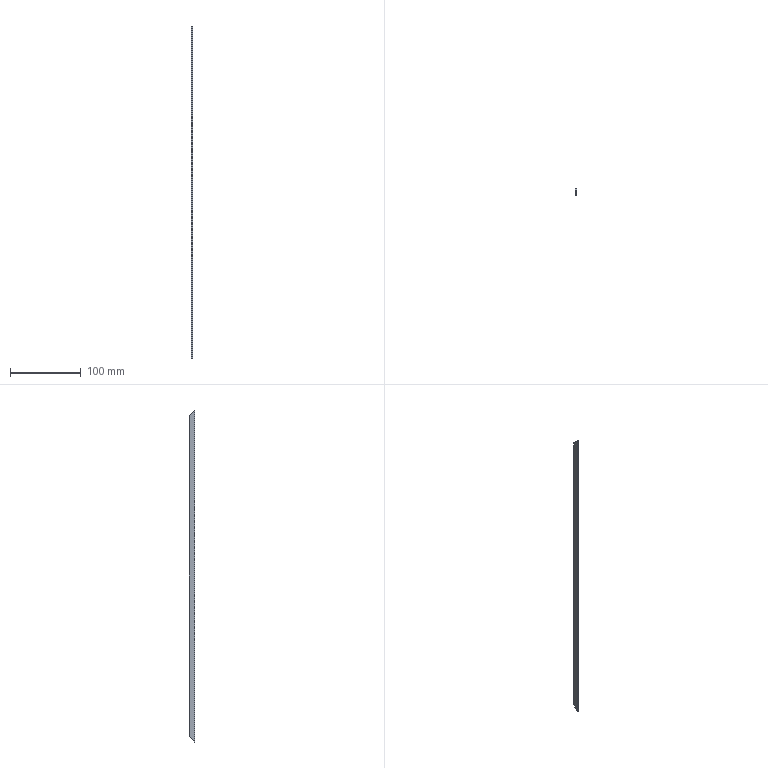Part | NX | features BREP 1 | 1 solid | 6 faces | box 1.5 x 8 x 468.1 mm | volume 5521 mm3 | plane 6
STEP:
#1=CARTESIAN_POINT('',(0.,8.,226.05));
#2=VERTEX_POINT('',#1);
#3=CARTESIAN_POINT('',(0.,8.,-226.05));
#4=VERTEX_POINT('',#3);
#5=CARTESIAN_POINT('',(0.,8.,234.05));
#6=DIRECTION('',(0.,0.,-1.));
#7=VECTOR('',#6,1000.);
#8=LINE('',#5,#7);
#9=EDGE_CURVE('',#2,#4,#8,.T.);
#10=ORIENTED_EDGE('',*,*,#9,.T.);
#11=CARTESIAN_POINT('',(0.,0.,-234.05));
#12=VERTEX_POINT('',#11);
#13=CARTESIAN_POINT('',(0.,8.,-226.05));
#14=DIRECTION('',(0.,-0.7071,-0.7071));
#15=VECTOR('',#14,1000.);
#16=LINE('',#13,#15);
#17=EDGE_CURVE('',#4,#12,#16,.T.);
#18=ORIENTED_EDGE('',*,*,#17,.T.);
#19=CARTESIAN_POINT('',(0.,0.,234.05));
#20=VERTEX_POINT('',#19);
#21=CARTESIAN_POINT('',(0.,0.,234.05));
#22=DIRECTION('',(0.,0.,-1.));
#23=VECTOR('',#22,1000.);
#24=LINE('',#21,#23);
#25=EDGE_CURVE('',#20,#12,#24,.T.);
#26=ORIENTED_EDGE('',*,*,#25,.F.);
#27=CARTESIAN_POINT('',(0.,0.,234.05));
#28=DIRECTION('',(0.,0.7071,-0.7071));
#29=VECTOR('',#28,1000.);
#30=LINE('',#27,#29);
#31=EDGE_CURVE('',#20,#2,#30,.T.);
#32=ORIENTED_EDGE('',*,*,#31,.T.);
#33=EDGE_LOOP('',(#10,#18,#26,#32));
#34=FACE_BOUND('',#33,.T.);
#35=CARTESIAN_POINT('',(0.,0.,234.05));
#36=DIRECTION('',(1.,0.,0.));
#37=DIRECTION('',(0.,1.,0.));
#38=AXIS2_PLACEMENT_3D('',#35,#36,#37);
#39=PLANE('',#38);
#40=ADVANCED_FACE('',(#34),#39,.F.);
#41=CARTESIAN_POINT('',(1.5,0.,-234.05));
#42=VERTEX_POINT('',#41);
#43=CARTESIAN_POINT('',(0.,0.,-234.05));
#44=DIRECTION('',(1.,0.,0.));
#45=VECTOR('',#44,1000.);
#46=LINE('',#43,#45);
#47=EDGE_CURVE('',#12,#42,#46,.T.);
#48=ORIENTED_EDGE('',*,*,#47,.T.);
#49=CARTESIAN_POINT('',(1.5,0.,234.05));
#50=VERTEX_POINT('',#49);
#51=CARTESIAN_POINT('',(1.5,0.,234.05));
#52=DIRECTION('',(0.,0.,-1.));
#53=VECTOR('',#52,1000.);
#54=LINE('',#51,#53);
#55=EDGE_CURVE('',#50,#42,#54,.T.);
#56=ORIENTED_EDGE('',*,*,#55,.F.);
#57=CARTESIAN_POINT('',(0.,0.,234.05));
#58=DIRECTION('',(1.,0.,0.));
#59=VECTOR('',#58,1000.);
#60=LINE('',#57,#59);
#61=EDGE_CURVE('',#20,#50,#60,.T.);
#62=ORIENTED_EDGE('',*,*,#61,.F.);
#63=ORIENTED_EDGE('',*,*,#25,.T.);
#64=EDGE_LOOP('',(#48,#56,#62,#63));
#65=FACE_BOUND('',#64,.T.);
#66=CARTESIAN_POINT('',(0.,0.,234.05));
#67=DIRECTION('',(0.,1.,0.));
#68=DIRECTION('',(1.,0.,0.));
#69=AXIS2_PLACEMENT_3D('',#66,#67,#68);
#70=PLANE('',#69);
#71=ADVANCED_FACE('',(#65),#70,.F.);
#72=ORIENTED_EDGE('',*,*,#55,.T.);
#73=CARTESIAN_POINT('',(1.5,8.,-226.05));
#74=VERTEX_POINT('',#73);
#75=CARTESIAN_POINT('',(1.5,8.,-226.05));
#76=DIRECTION('',(0.,0.7071,0.7071));
#77=VECTOR('',#76,1000.);
#78=LINE('',#75,#77);
#79=EDGE_CURVE('',#42,#74,#78,.T.);
#80=ORIENTED_EDGE('',*,*,#79,.T.);
#81=CARTESIAN_POINT('',(1.5,8.,226.05));
#82=VERTEX_POINT('',#81);
#83=CARTESIAN_POINT('',(1.5,8.,234.05));
#84=DIRECTION('',(0.,0.,-1.));
#85=VECTOR('',#84,1000.);
#86=LINE('',#83,#85);
#87=EDGE_CURVE('',#82,#74,#86,.T.);
#88=ORIENTED_EDGE('',*,*,#87,.F.);
#89=CARTESIAN_POINT('',(1.5,0.,234.05));
#90=DIRECTION('',(0.,-0.7071,0.7071));
#91=VECTOR('',#90,1000.);
#92=LINE('',#89,#91);
#93=EDGE_CURVE('',#82,#50,#92,.T.);
#94=ORIENTED_EDGE('',*,*,#93,.T.);
#95=EDGE_LOOP('',(#72,#80,#88,#94));
#96=FACE_BOUND('',#95,.T.);
#97=CARTESIAN_POINT('',(1.5,0.,234.05));
#98=DIRECTION('',(-1.,0.,0.));
#99=DIRECTION('',(0.,0.,1.));
#100=AXIS2_PLACEMENT_3D('',#97,#98,#99);
#101=PLANE('',#100);
#102=ADVANCED_FACE('',(#96),#101,.F.);
#103=ORIENTED_EDGE('',*,*,#87,.T.);
#104=CARTESIAN_POINT('',(0.,8.,-226.05));
#105=DIRECTION('',(-1.,0.,0.));
#106=VECTOR('',#105,1000.);
#107=LINE('',#104,#106);
#108=EDGE_CURVE('',#74,#4,#107,.T.);
#109=ORIENTED_EDGE('',*,*,#108,.T.);
#110=ORIENTED_EDGE('',*,*,#9,.F.);
#111=CARTESIAN_POINT('',(0.,8.,226.05));
#112=DIRECTION('',(1.,0.,0.));
#113=VECTOR('',#112,1000.);
#114=LINE('',#111,#113);
#115=EDGE_CURVE('',#2,#82,#114,.T.);
#116=ORIENTED_EDGE('',*,*,#115,.T.);
#117=EDGE_LOOP('',(#103,#109,#110,#116));
#118=FACE_BOUND('',#117,.T.);
#119=CARTESIAN_POINT('',(0.,8.,234.05));
#120=DIRECTION('',(0.,-1.,0.));
#121=DIRECTION('',(0.,0.,-1.));
#122=AXIS2_PLACEMENT_3D('',#119,#120,#121);
#123=PLANE('',#122);
#124=ADVANCED_FACE('',(#118),#123,.F.);
#125=ORIENTED_EDGE('',*,*,#79,.F.);
#126=ORIENTED_EDGE('',*,*,#47,.F.);
#127=ORIENTED_EDGE('',*,*,#17,.F.);
#128=ORIENTED_EDGE('',*,*,#108,.F.);
#129=EDGE_LOOP('',(#125,#126,#127,#128));
#130=FACE_BOUND('',#129,.T.);
#131=CARTESIAN_POINT('',(0.,8.,-226.05));
#132=DIRECTION('',(0.,0.7071,-0.7071));
#133=DIRECTION('',(-1.,0.,0.));
#134=AXIS2_PLACEMENT_3D('',#131,#132,#133);
#135=PLANE('',#134);
#136=ADVANCED_FACE('',(#130),#135,.T.);
#137=ORIENTED_EDGE('',*,*,#93,.F.);
#138=ORIENTED_EDGE('',*,*,#115,.F.);
#139=ORIENTED_EDGE('',*,*,#31,.F.);
#140=ORIENTED_EDGE('',*,*,#61,.T.);
#141=EDGE_LOOP('',(#137,#138,#139,#140));
#142=FACE_BOUND('',#141,.T.);
#143=CARTESIAN_POINT('',(0.,0.,234.05));
#144=DIRECTION('',(0.,-0.7071,-0.7071));
#145=DIRECTION('',(0.,0.7071,-0.7071));
#146=AXIS2_PLACEMENT_3D('',#143,#144,#145);
#147=PLANE('',#146);
#148=ADVANCED_FACE('',(#142),#147,.F.);
#149=CLOSED_SHELL('',(#40,#71,#102,#124,#136,#148));
#150=MANIFOLD_SOLID_BREP('',#149);
#151=(LENGTH_UNIT()NAMED_UNIT(*)SI_UNIT(.MILLI.,.METRE.));
#152=UNCERTAINTY_MEASURE_WITH_UNIT(LENGTH_MEASURE(0.00001),#151,'','');
#153=(NAMED_UNIT(*)PLANE_ANGLE_UNIT()SI_UNIT($,.RADIAN.));
#154=(NAMED_UNIT(*)SI_UNIT($,.STERADIAN.)SOLID_ANGLE_UNIT());
#155=(GEOMETRIC_REPRESENTATION_CONTEXT(3)GLOBAL_UNCERTAINTY_ASSIGNED_CONTEXT((#152))GLOBAL_UNIT_ASSIGNED_CONTEXT((#151,#153,#154))REPRESENTATION_CONTEXT('',''));
#156=ADVANCED_BREP_SHAPE_REPRESENTATION('',(#150),#155);